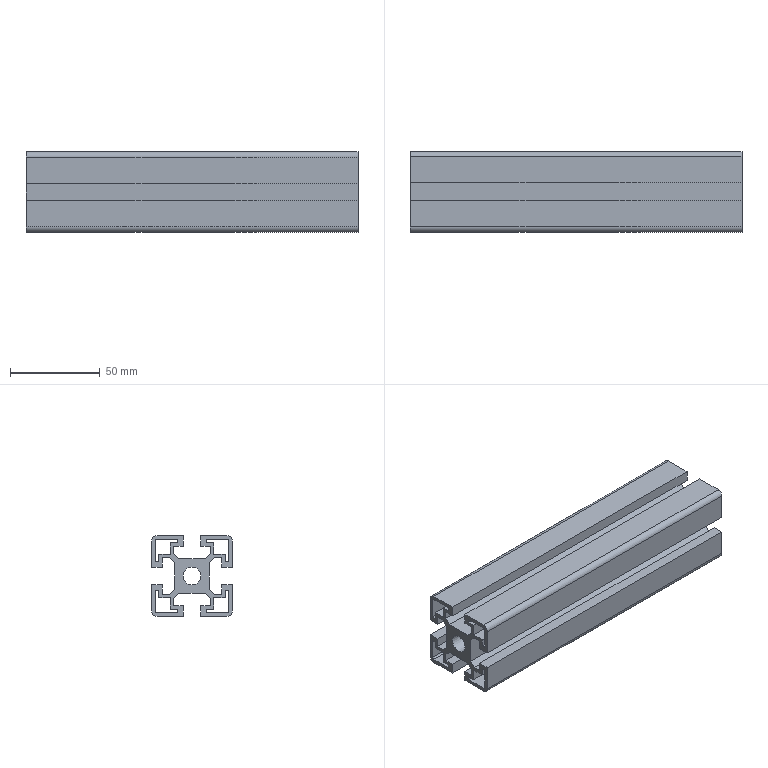Part | STEP file | 1_9 | 1 solid | 87 faces | box 185 x 45 x 45 mm | volume 151282 mm3 | plane 78 | cylinder 9 | commonest cylinder face diameters 2 x4 6 x4 10 x1